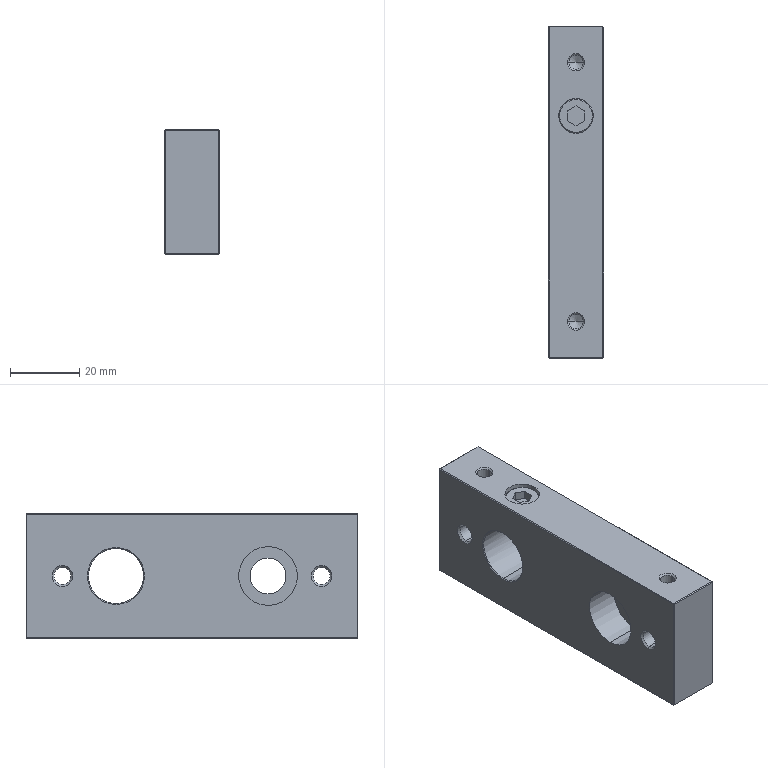Part | STEP file | TR_32x10-2 | 1 solid | 65 faces | box 16 x 96 x 36 mm | volume 48259 mm3 | plane 27 | cone 22 | cylinder 16 | commonest cylinder face diameters 4.134 x4 4.917 x4 10 x2 10.4 x2 16 x2 17 x2